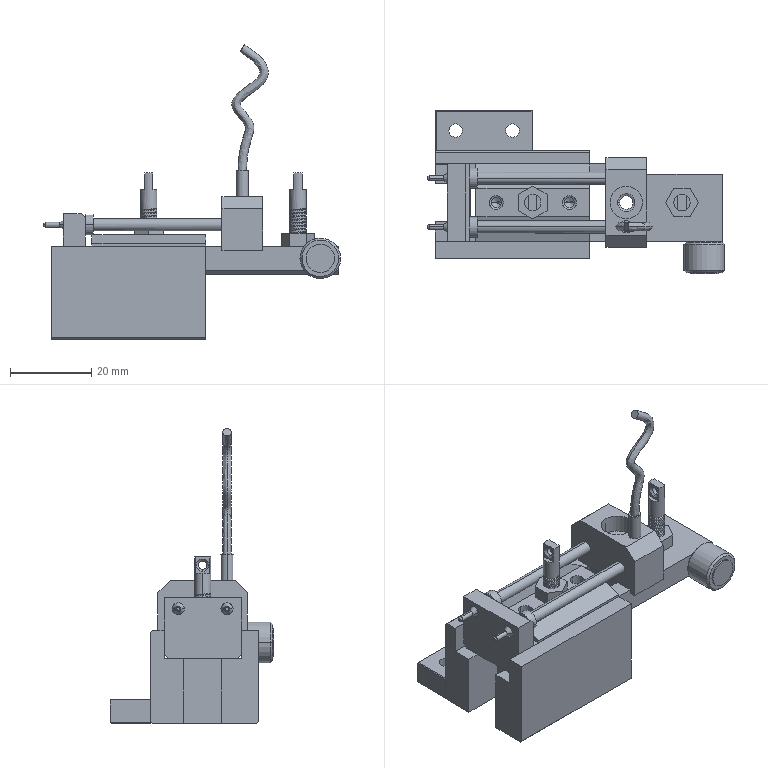Part | NX | 13 solids | 360 faces | box 73.15 x 40.25 x 72.548 mm | volume 31241 mm3 | cylinder 152 | plane 126 | cone 64 | spline 18 | commonest cylinder face diameters 4 x58 3 x28 3.3 x16 2.5 x14 3.5 x6 1 x4